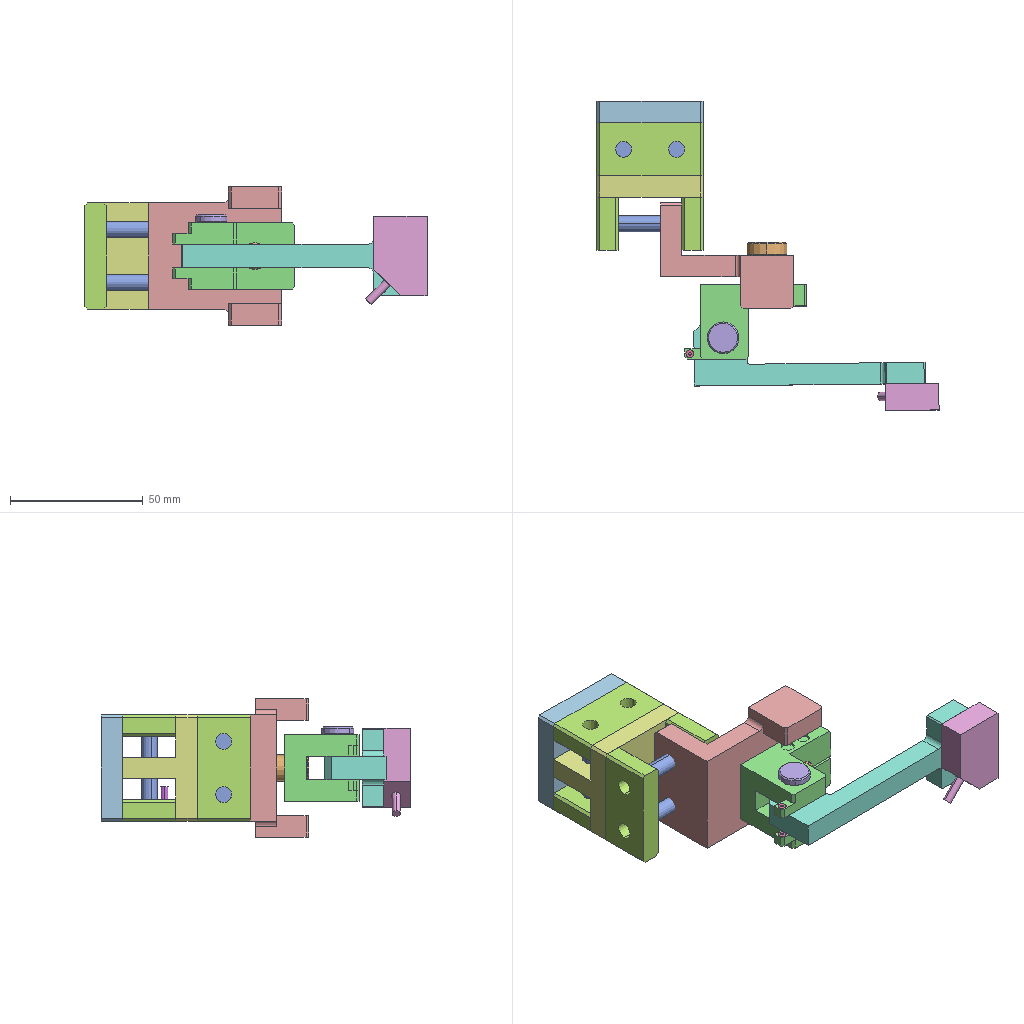Assembly | SolidWorks | 13 different items | 20 placed | box 129 x 116 x 52 mm
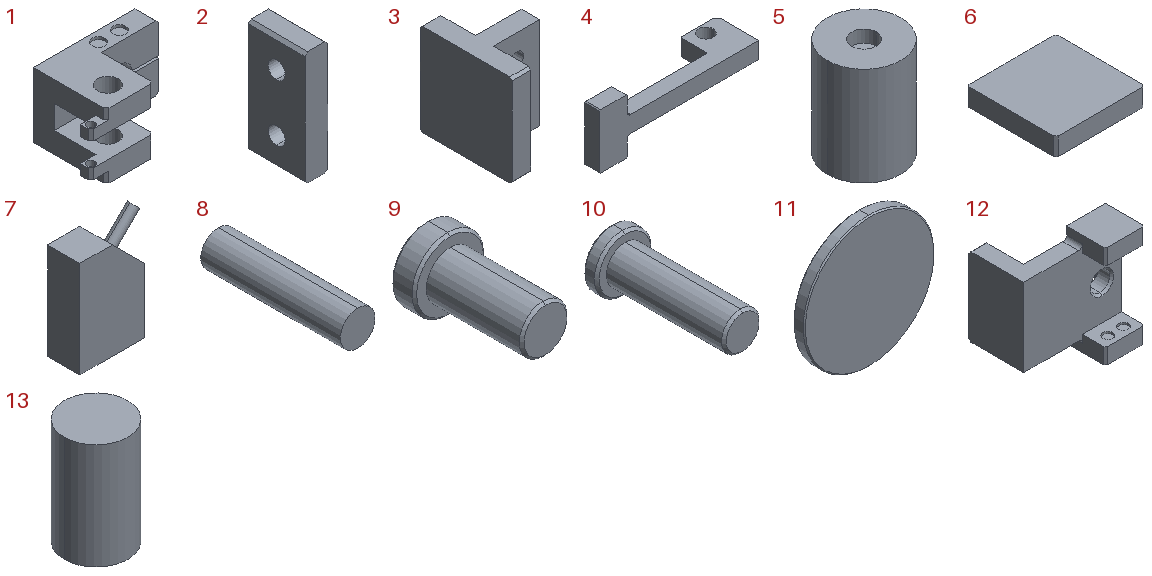Parts list (item | quantity | size | volume | features):
1 | x1 | 46 x 28 x 25 mm | 12240 mm3 | features ICE 8, Chamfer 2, Extrusion 1
2 | x4 | 8 x 20 x 40 mm | 5908 mm3 | features Chamfer 1, Extrusion 1, ICE 1
3 | x1 | 28 x 40 x 40 mm | 18732 mm3 | features ICE 2, Chamfer 1, Extrusion 1
4 | x1 | 87 x 23 x 30 mm | 11014 mm3 | features Chamfer 2, Fillet 2, ICE 2, Cut 1, Extrusion 1, MoveFace 1
5 | x2 | 3 x 3 x 4 mm | 27.685 mm3 | features ICE 2, Extrusion 1
6 | x1 | 40 x 40 x 8 mm | 12784 mm3 | features Chamfer 1, Extrusion 1
7 | x1 | 23.098 x 10 x 33.285 mm | 5579 mm3 | features Chamfer 1, Extrusion 1, ICE 1
8 | x4 | 6 x 24 x 6 mm | 678.584 mm3 | features Extrusion 1
9 | x1 | 15 x 25 x 15 mm | 2439 mm3 | features Chamfer 1, Extrusion 1, ICE 1
10 | x1 | 12 x 28 x 12 mm | 1584 mm3 | features Chamfer 1, Extrusion 1, ICE 1
11 | x1 | 116 x 10 x 116 mm | 105321 mm3 | features Chamfer 1, Extrusion 1
12 | x1 | 50 x 40 x 52 mm | 27409 mm3 | features ICE 5, Chamfer 3, Cut 1, Extrusion 1, Fillet 1
13 | x1 | 3 x 3 x 5 mm | 35.343 mm3 | features Extrusion 1
Mates (type | each side: item.copy, entity, surface, feature):
Concentric | 12.1 face cylinder Cut-Extrude1 | 9.1 face cylinder Boss-Extrude1
Parallel | 12.1 face plane Boss-Extrude1 | 9.1 plane
Coincident | 12.1 face plane Boss-Extrude1 | 9.1 face plane Boss-Extrude2
Concentric | 4.1 face cylinder Cut-Extrude1 | 10.1 face cylinder Boss-Extrude1
Coincident | 7.1 face plane Boss-Extrude1 | 4.1 face plane Boss-Extrude1
DistanceDim | 7.1 face plane Boss-Extrude1 | 4.1 face plane Boss-Extrude1
Width | 7.1 face plane Boss-Extrude1 | 7.1 face plane Boss-Extrude1 | 4.1 face plane Boss-Extrude3 | 4.1 face plane Boss-Extrude3
Coincident | 2.1 face plane Boss-Extrude1 | 2.2 face plane Boss-Extrude1 | 2 times
DistanceDim | 2.1 face plane Boss-Extrude1 | 12.1 face plane Boss-Extrude1
Coincident | 12.1 face plane Boss-Extrude1 | 2.2 face plane Boss-Extrude1
LimitDistanceDim | 12.1 face plane Boss-Extrude4 | 2.2 face plane Boss-Extrude1
Coincident | 8.1 face plane Boss-Extrude1 | 8.2 face plane Boss-Extrude1
Coincident | 8.1 face plane Boss-Extrude1 | 2.1 face plane Boss-Extrude1
Concentric | 8.1 face cylinder Boss-Extrude1 | 2.1 face cylinder Cut-Extrude1
Concentric | 8.2 face cylinder Boss-Extrude1 | 2.2 face cylinder Cut-Extrude1
Concentric | 9.1 face cylinder Boss-Extrude1 | 1.1 face cylinder Cut-Extrude1
Concentric | 10.1 face cylinder Boss-Extrude1 | 1.1 face cylinder Cut-Extrude3
Parallel | 12.1 face plane Boss-Extrude2 | 1.1 face plane Boss-Extrude1
Coincident | 10.1 face plane Boss-Extrude2 | 1.1 face plane Boss-Extrude1
Width | 4.1 face plane Boss-Extrude1 | 4.1 face plane Boss-Extrude1 | 1.1 face plane Boss-Extrude2 | 1.1 face plane Boss-Extrude2
Concentric | 12.1 edge | 1.1 face cylinder Cut-Extrude4
Concentric | 1.1 face cylinder Cut-Extrude6 | 5.1 face cylinder Cut-Extrude2
Concentric | 1.1 face cylinder Cut-Extrude6 | 5.2 face cylinder Boss-Extrude1
Coincident | 1.1 face plane Boss-Extrude3 | 5.1 face plane Boss-Extrude1
Coincident | 1.1 face plane Boss-Extrude2 | 5.2 face plane Boss-Extrude1
Concentric | assembly face | assembly face
Coincident | assembly face | assembly face | 2 times
Concentric | 2.3 face cylinder Cut-Extrude1 | 8.3 face cylinder Boss-Extrude1
Concentric | 2.4 face cylinder Cut-Extrude1 | 8.4 face cylinder Boss-Extrude1
Coincident | 2.3 face plane Boss-Extrude1 | 8.3 face plane Boss-Extrude1
Coincident | 2.4 face plane Boss-Extrude1 | 2.3 face plane Boss-Extrude1 | 2 times
Coincident | 8.4 face plane Boss-Extrude1 | 8.3 face plane Boss-Extrude1
Coincident | 2.4 face plane Boss-Extrude1 | 8.4 edge
Coincident | 2.2 face plane Boss-Extrude1 | 2.4 face plane Boss-Extrude1
Coincident | 6.1 face plane Boss-Extrude1 | 2.4 face plane Boss-Extrude1 | 3 times
Coincident | 2.4 face plane Boss-Extrude1 | 3.1 face plane Boss-Extrude1
Coincident | 6.1 face plane Boss-Extrude1 | 3.1 face plane Boss-Extrude2
Coincident | 2.2 face plane Boss-Extrude1 | 3.1 face plane Boss-Extrude1 | 3 times
Coincident | 2.1 face plane Boss-Extrude1 | 3.1 face plane Boss-Extrude1
Coincident | 2.4 face plane Boss-Extrude1 | 13.1 face plane Boss-Extrude1